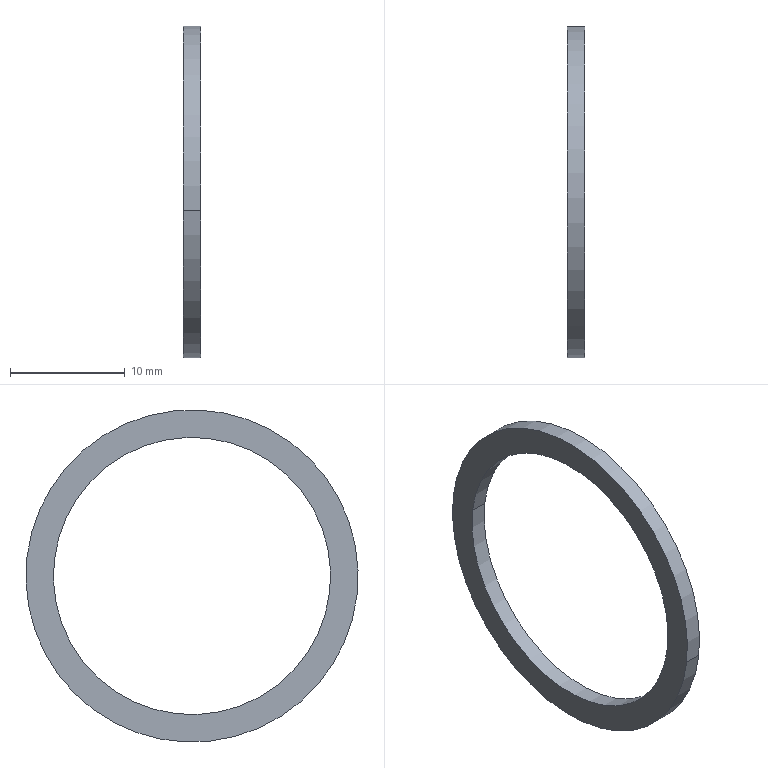Part | SolidWorks | features BaseBody 1 | 1 solid | 6 faces | box 1.5 x 29 x 29 mm | volume 300.839 mm3 | cylinder 4 | plane 2 | commonest cylinder face diameters 24.2 x2 29 x2
STEP:
#1=CARTESIAN_POINT('',(0.,110.022,-14.627));
#2=VERTEX_POINT('',#1);
#3=CARTESIAN_POINT('',(0.,85.978,-17.373));
#4=VERTEX_POINT('',#3);
#5=CARTESIAN_POINT('',(0.,98.,-16.));
#6=DIRECTION('',(1.,0.,0.));
#7=DIRECTION('',(0.,-0.9935,-0.1135));
#8=AXIS2_PLACEMENT_3D('',#5,#6,#7);
#9=CIRCLE('',#8,12.1);
#10=EDGE_CURVE('',#2,#4,#9,.T.);
#11=ORIENTED_EDGE('',*,*,#10,.T.);
#12=CARTESIAN_POINT('',(-1.5,85.978,-17.373));
#13=VERTEX_POINT('',#12);
#14=CARTESIAN_POINT('',(0.,85.978,-17.373));
#15=DIRECTION('',(-1.,0.,0.));
#16=VECTOR('',#15,1000.);
#17=LINE('',#14,#16);
#18=EDGE_CURVE('',#4,#13,#17,.T.);
#19=ORIENTED_EDGE('',*,*,#18,.T.);
#20=CARTESIAN_POINT('',(-1.5,110.022,-14.627));
#21=VERTEX_POINT('',#20);
#22=CARTESIAN_POINT('',(-1.5,98.,-16.));
#23=DIRECTION('',(1.,0.,0.));
#24=DIRECTION('',(0.,-0.9935,-0.1135));
#25=AXIS2_PLACEMENT_3D('',#22,#23,#24);
#26=CIRCLE('',#25,12.1);
#27=EDGE_CURVE('',#21,#13,#26,.T.);
#28=ORIENTED_EDGE('',*,*,#27,.F.);
#29=CARTESIAN_POINT('',(0.,110.022,-14.627));
#30=DIRECTION('',(-1.,0.,0.));
#31=VECTOR('',#30,1000.);
#32=LINE('',#29,#31);
#33=EDGE_CURVE('',#2,#21,#32,.T.);
#34=ORIENTED_EDGE('',*,*,#33,.F.);
#35=EDGE_LOOP('',(#11,#19,#28,#34));
#36=FACE_OUTER_BOUND('',#35,.T.);
#37=CARTESIAN_POINT('',(0.,98.,-16.));
#38=DIRECTION('',(-1.,0.,0.));
#39=DIRECTION('',(0.,0.9935,0.1135));
#40=AXIS2_PLACEMENT_3D('',#37,#38,#39);
#41=CYLINDRICAL_SURFACE('',#40,12.1);
#42=ADVANCED_FACE('',(#36),#41,.F.);
#43=CARTESIAN_POINT('',(0.,83.594,-17.645));
#44=VERTEX_POINT('',#43);
#45=CARTESIAN_POINT('',(0.,112.406,-14.355));
#46=VERTEX_POINT('',#45);
#47=CARTESIAN_POINT('',(0.,98.,-16.));
#48=DIRECTION('',(1.,0.,0.));
#49=DIRECTION('',(0.,-0.9935,-0.1135));
#50=AXIS2_PLACEMENT_3D('',#47,#48,#49);
#51=CIRCLE('',#50,14.5);
#52=EDGE_CURVE('',#44,#46,#51,.T.);
#53=ORIENTED_EDGE('',*,*,#52,.F.);
#54=CARTESIAN_POINT('',(-1.5,83.594,-17.645));
#55=VERTEX_POINT('',#54);
#56=CARTESIAN_POINT('',(0.,83.594,-17.645));
#57=DIRECTION('',(-1.,0.,0.));
#58=VECTOR('',#57,1000.);
#59=LINE('',#56,#58);
#60=EDGE_CURVE('',#44,#55,#59,.T.);
#61=ORIENTED_EDGE('',*,*,#60,.T.);
#62=CARTESIAN_POINT('',(-1.5,112.406,-14.355));
#63=VERTEX_POINT('',#62);
#64=CARTESIAN_POINT('',(-1.5,98.,-16.));
#65=DIRECTION('',(1.,0.,0.));
#66=DIRECTION('',(0.,-0.9935,-0.1135));
#67=AXIS2_PLACEMENT_3D('',#64,#65,#66);
#68=CIRCLE('',#67,14.5);
#69=EDGE_CURVE('',#55,#63,#68,.T.);
#70=ORIENTED_EDGE('',*,*,#69,.T.);
#71=CARTESIAN_POINT('',(0.,112.406,-14.355));
#72=DIRECTION('',(-1.,0.,0.));
#73=VECTOR('',#72,1000.);
#74=LINE('',#71,#73);
#75=EDGE_CURVE('',#46,#63,#74,.T.);
#76=ORIENTED_EDGE('',*,*,#75,.F.);
#77=EDGE_LOOP('',(#53,#61,#70,#76));
#78=FACE_OUTER_BOUND('',#77,.T.);
#79=CARTESIAN_POINT('',(0.,98.,-16.));
#80=DIRECTION('',(-1.,0.,0.));
#81=DIRECTION('',(0.,0.9935,0.1135));
#82=AXIS2_PLACEMENT_3D('',#79,#80,#81);
#83=CYLINDRICAL_SURFACE('',#82,14.5);
#84=ADVANCED_FACE('',(#78),#83,.T.);
#85=CARTESIAN_POINT('',(0.,98.,-16.));
#86=DIRECTION('',(1.,0.,0.));
#87=DIRECTION('',(0.,-0.9935,-0.1135));
#88=AXIS2_PLACEMENT_3D('',#85,#86,#87);
#89=CIRCLE('',#88,14.5);
#90=EDGE_CURVE('',#46,#44,#89,.T.);
#91=ORIENTED_EDGE('',*,*,#90,.T.);
#92=ORIENTED_EDGE('',*,*,#52,.T.);
#93=EDGE_LOOP('',(#91,#92));
#94=FACE_OUTER_BOUND('',#93,.T.);
#95=ORIENTED_EDGE('',*,*,#10,.F.);
#96=CARTESIAN_POINT('',(0.,98.,-16.));
#97=DIRECTION('',(1.,0.,0.));
#98=DIRECTION('',(0.,-0.9935,-0.1135));
#99=AXIS2_PLACEMENT_3D('',#96,#97,#98);
#100=CIRCLE('',#99,12.1);
#101=EDGE_CURVE('',#4,#2,#100,.T.);
#102=ORIENTED_EDGE('',*,*,#101,.F.);
#103=EDGE_LOOP('',(#95,#102));
#104=FACE_BOUND('',#103,.T.);
#105=CARTESIAN_POINT('',(0.,98.,-16.));
#106=DIRECTION('',(1.,0.,0.));
#107=DIRECTION('',(0.,-0.9935,-0.1135));
#108=AXIS2_PLACEMENT_3D('',#105,#106,#107);
#109=PLANE('',#108);
#110=ADVANCED_FACE('',(#94,#104),#109,.T.);
#111=CARTESIAN_POINT('',(-1.5,98.,-16.));
#112=DIRECTION('',(1.,0.,0.));
#113=DIRECTION('',(0.,-0.9935,-0.1135));
#114=AXIS2_PLACEMENT_3D('',#111,#112,#113);
#115=CIRCLE('',#114,14.5);
#116=EDGE_CURVE('',#63,#55,#115,.T.);
#117=ORIENTED_EDGE('',*,*,#116,.F.);
#118=ORIENTED_EDGE('',*,*,#69,.F.);
#119=EDGE_LOOP('',(#117,#118));
#120=FACE_OUTER_BOUND('',#119,.T.);
#121=ORIENTED_EDGE('',*,*,#27,.T.);
#122=CARTESIAN_POINT('',(-1.5,98.,-16.));
#123=DIRECTION('',(1.,0.,0.));
#124=DIRECTION('',(0.,-0.9935,-0.1135));
#125=AXIS2_PLACEMENT_3D('',#122,#123,#124);
#126=CIRCLE('',#125,12.1);
#127=EDGE_CURVE('',#13,#21,#126,.T.);
#128=ORIENTED_EDGE('',*,*,#127,.T.);
#129=EDGE_LOOP('',(#121,#128));
#130=FACE_BOUND('',#129,.T.);
#131=CARTESIAN_POINT('',(-1.5,98.,-16.));
#132=DIRECTION('',(1.,0.,0.));
#133=DIRECTION('',(0.,-0.9935,-0.1135));
#134=AXIS2_PLACEMENT_3D('',#131,#132,#133);
#135=PLANE('',#134);
#136=ADVANCED_FACE('',(#120,#130),#135,.F.);
#137=ORIENTED_EDGE('',*,*,#60,.F.);
#138=ORIENTED_EDGE('',*,*,#90,.F.);
#139=ORIENTED_EDGE('',*,*,#75,.T.);
#140=ORIENTED_EDGE('',*,*,#116,.T.);
#141=EDGE_LOOP('',(#137,#138,#139,#140));
#142=FACE_OUTER_BOUND('',#141,.T.);
#143=CARTESIAN_POINT('',(0.,98.,-16.));
#144=DIRECTION('',(-1.,0.,0.));
#145=DIRECTION('',(0.,0.9935,0.1135));
#146=AXIS2_PLACEMENT_3D('',#143,#144,#145);
#147=CYLINDRICAL_SURFACE('',#146,14.5);
#148=ADVANCED_FACE('',(#142),#147,.T.);
#149=ORIENTED_EDGE('',*,*,#18,.F.);
#150=ORIENTED_EDGE('',*,*,#101,.T.);
#151=ORIENTED_EDGE('',*,*,#33,.T.);
#152=ORIENTED_EDGE('',*,*,#127,.F.);
#153=EDGE_LOOP('',(#149,#150,#151,#152));
#154=FACE_OUTER_BOUND('',#153,.T.);
#155=CARTESIAN_POINT('',(0.,98.,-16.));
#156=DIRECTION('',(-1.,0.,0.));
#157=DIRECTION('',(0.,0.9935,0.1135));
#158=AXIS2_PLACEMENT_3D('',#155,#156,#157);
#159=CYLINDRICAL_SURFACE('',#158,12.1);
#160=ADVANCED_FACE('',(#154),#159,.F.);
#161=CLOSED_SHELL('',(#42,#84,#110,#136,#148,#160));
#162=MANIFOLD_SOLID_BREP('',#161);
#163=CARTESIAN_POINT('',(0.,0.,0.));
#164=DIRECTION('',(0.,0.,1.));
#165=DIRECTION('',(1.,0.,0.));
#166=AXIS2_PLACEMENT_3D('',#163,#164,#165);
#167=(LENGTH_UNIT()NAMED_UNIT(*)SI_UNIT(.MILLI.,.METRE.));
#168=UNCERTAINTY_MEASURE_WITH_UNIT(LENGTH_MEASURE(0.00001),#167,'','');
#169=(NAMED_UNIT(*)PLANE_ANGLE_UNIT()SI_UNIT($,.RADIAN.));
#170=(NAMED_UNIT(*)SI_UNIT($,.STERADIAN.)SOLID_ANGLE_UNIT());
#171=(GEOMETRIC_REPRESENTATION_CONTEXT(3)GLOBAL_UNCERTAINTY_ASSIGNED_CONTEXT((#168))GLOBAL_UNIT_ASSIGNED_CONTEXT((#167,#169,#170))REPRESENTATION_CONTEXT('',''));
#172=ADVANCED_BREP_SHAPE_REPRESENTATION('',(#162,#166),#171);